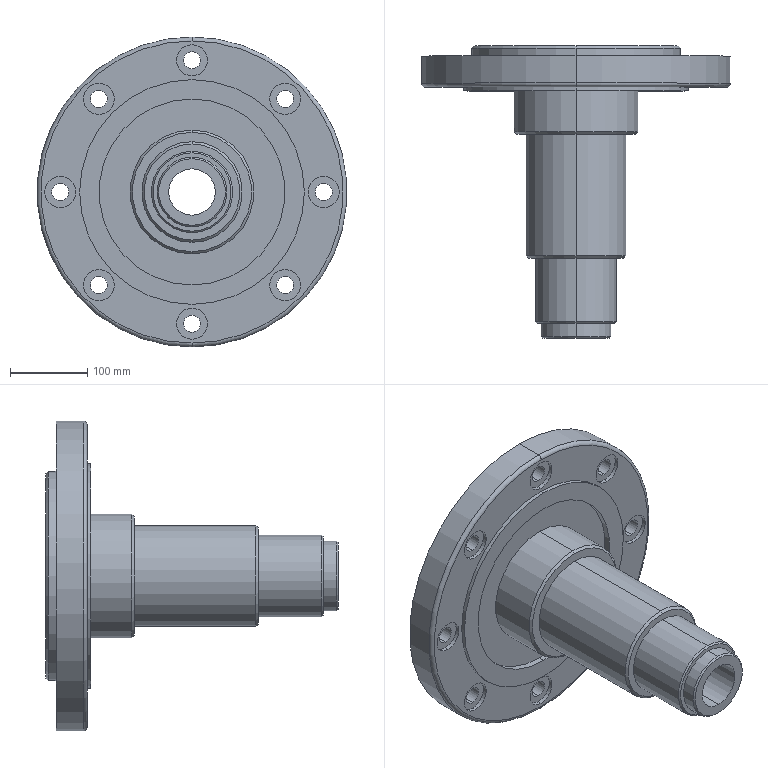Part | SolidWorks | features ICE 5, Chamfer 2, Revolution 1 | 1 solid | 88 faces | box 400 x 377 x 400 mm | volume 7916207 mm3 | cylinder 54 | plane 18 | cone 14 | torus 2 | commonest cylinder face diameters 22 x16 40 x16 90 x4 60 x2 105 x2 120 x2